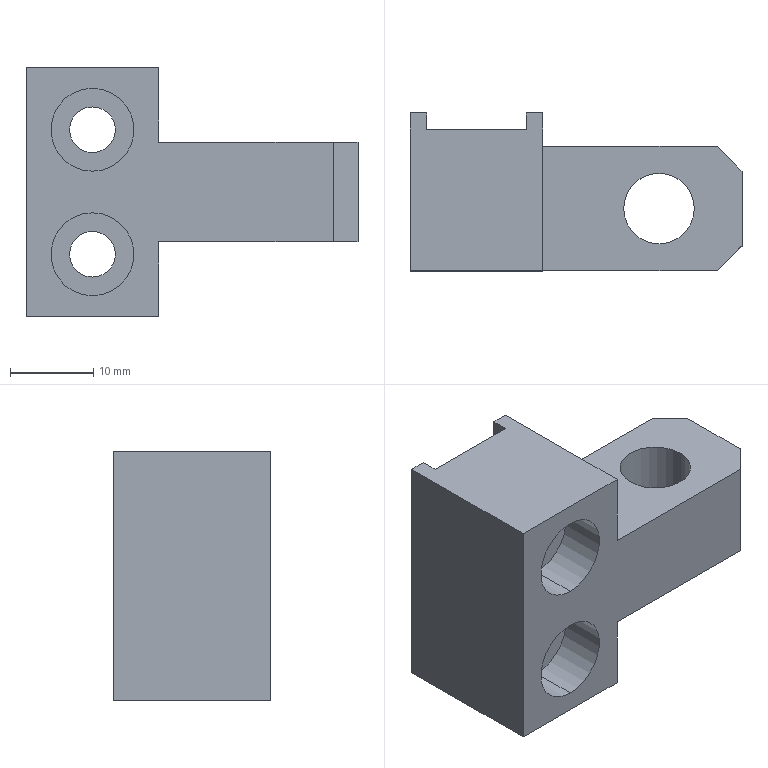Part | STEP file | PN_0027 | 1 solid | 28 faces | box 40 x 19 x 30 mm | volume 10499 mm3 | plane 18 | cylinder 10 | commonest cylinder face diameters 5.5 x4 10 x4 8.5 x2